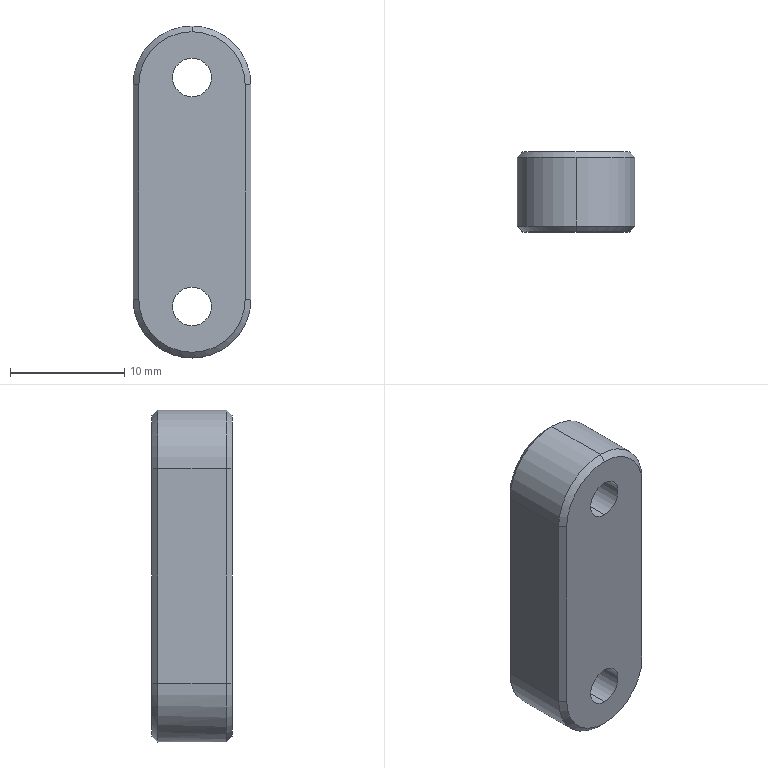Part | SolidWorks | features Fillet 2, ICE 2, Chamfer 1, Extrusion 1, HoleWzd 1 | 1 solid | 27 faces | box 10.3 x 7 x 29 mm | volume 1657 mm3 | cylinder 11 | plane 10 | cone 6 | commonest cylinder face diameters 3.4 x4 6 x4 10.3 x3
STEP:
#1=CARTESIAN_POINT('',(0.,0.1,21.5));
#2=VERTEX_POINT('',#1);
#3=CARTESIAN_POINT('',(0.,0.1,27.5));
#4=VERTEX_POINT('',#3);
#5=CARTESIAN_POINT('',(0.,0.1,24.5));
#6=DIRECTION('',(0.,1.,0.));
#7=DIRECTION('',(0.,0.,1.));
#8=AXIS2_PLACEMENT_3D('',#5,#6,#7);
#9=CIRCLE('',#8,3.);
#10=EDGE_CURVE('',#2,#4,#9,.T.);
#11=ORIENTED_EDGE('',*,*,#10,.F.);
#12=CARTESIAN_POINT('',(0.,3.5,21.5));
#13=VERTEX_POINT('',#12);
#14=CARTESIAN_POINT('',(0.,3.5,21.5));
#15=DIRECTION('',(0.,1.,0.));
#16=VECTOR('',#15,1000.);
#17=LINE('',#14,#16);
#18=EDGE_CURVE('',#2,#13,#17,.T.);
#19=ORIENTED_EDGE('',*,*,#18,.T.);
#20=CARTESIAN_POINT('',(0.,3.5,27.5));
#21=VERTEX_POINT('',#20);
#22=CARTESIAN_POINT('',(0.,3.5,24.5));
#23=DIRECTION('',(0.,1.,0.));
#24=DIRECTION('',(0.,0.,1.));
#25=AXIS2_PLACEMENT_3D('',#22,#23,#24);
#26=CIRCLE('',#25,3.);
#27=EDGE_CURVE('',#13,#21,#26,.T.);
#28=ORIENTED_EDGE('',*,*,#27,.T.);
#29=CARTESIAN_POINT('',(0.,3.5,27.5));
#30=DIRECTION('',(0.,1.,0.));
#31=VECTOR('',#30,1000.);
#32=LINE('',#29,#31);
#33=EDGE_CURVE('',#4,#21,#32,.T.);
#34=ORIENTED_EDGE('',*,*,#33,.F.);
#35=EDGE_LOOP('',(#11,#19,#28,#34));
#36=FACE_OUTER_BOUND('',#35,.T.);
#37=CARTESIAN_POINT('',(0.,3.5,24.5));
#38=DIRECTION('',(0.,1.,0.));
#39=DIRECTION('',(0.,0.,1.));
#40=AXIS2_PLACEMENT_3D('',#37,#38,#39);
#41=CYLINDRICAL_SURFACE('',#40,3.);
#42=ADVANCED_FACE('',(#36),#41,.F.);
#43=CARTESIAN_POINT('',(0.,-3.5,22.8));
#44=VERTEX_POINT('',#43);
#45=CARTESIAN_POINT('',(0.,-3.5,26.2));
#46=VERTEX_POINT('',#45);
#47=CARTESIAN_POINT('',(0.,-3.5,24.5));
#48=DIRECTION('',(0.,1.,0.));
#49=DIRECTION('',(0.,0.,1.));
#50=AXIS2_PLACEMENT_3D('',#47,#48,#49);
#51=CIRCLE('',#50,1.7);
#52=EDGE_CURVE('',#44,#46,#51,.T.);
#53=ORIENTED_EDGE('',*,*,#52,.F.);
#54=CARTESIAN_POINT('',(0.,0.1,22.8));
#55=VERTEX_POINT('',#54);
#56=CARTESIAN_POINT('',(0.,3.5,22.8));
#57=DIRECTION('',(0.,1.,0.));
#58=VECTOR('',#57,1000.);
#59=LINE('',#56,#58);
#60=EDGE_CURVE('',#44,#55,#59,.T.);
#61=ORIENTED_EDGE('',*,*,#60,.T.);
#62=CARTESIAN_POINT('',(0.,0.1,26.2));
#63=VERTEX_POINT('',#62);
#64=CARTESIAN_POINT('',(0.,0.1,24.5));
#65=DIRECTION('',(0.,1.,0.));
#66=DIRECTION('',(0.,0.,1.));
#67=AXIS2_PLACEMENT_3D('',#64,#65,#66);
#68=CIRCLE('',#67,1.7);
#69=EDGE_CURVE('',#55,#63,#68,.T.);
#70=ORIENTED_EDGE('',*,*,#69,.T.);
#71=CARTESIAN_POINT('',(0.,3.5,26.2));
#72=DIRECTION('',(0.,1.,0.));
#73=VECTOR('',#72,1000.);
#74=LINE('',#71,#73);
#75=EDGE_CURVE('',#46,#63,#74,.T.);
#76=ORIENTED_EDGE('',*,*,#75,.F.);
#77=EDGE_LOOP('',(#53,#61,#70,#76));
#78=FACE_OUTER_BOUND('',#77,.T.);
#79=CARTESIAN_POINT('',(0.,3.5,24.5));
#80=DIRECTION('',(0.,1.,0.));
#81=DIRECTION('',(0.,0.,1.));
#82=AXIS2_PLACEMENT_3D('',#79,#80,#81);
#83=CYLINDRICAL_SURFACE('',#82,1.7);
#84=ADVANCED_FACE('',(#78),#83,.F.);
#85=CARTESIAN_POINT('',(0.,0.1,1.5));
#86=VERTEX_POINT('',#85);
#87=CARTESIAN_POINT('',(0.,0.1,7.5));
#88=VERTEX_POINT('',#87);
#89=CARTESIAN_POINT('',(0.,0.1,4.5));
#90=DIRECTION('',(0.,1.,0.));
#91=DIRECTION('',(0.,0.,1.));
#92=AXIS2_PLACEMENT_3D('',#89,#90,#91);
#93=CIRCLE('',#92,3.);
#94=EDGE_CURVE('',#86,#88,#93,.T.);
#95=ORIENTED_EDGE('',*,*,#94,.F.);
#96=CARTESIAN_POINT('',(0.,3.5,1.5));
#97=VERTEX_POINT('',#96);
#98=CARTESIAN_POINT('',(0.,3.5,1.5));
#99=DIRECTION('',(0.,1.,0.));
#100=VECTOR('',#99,1000.);
#101=LINE('',#98,#100);
#102=EDGE_CURVE('',#86,#97,#101,.T.);
#103=ORIENTED_EDGE('',*,*,#102,.T.);
#104=CARTESIAN_POINT('',(0.,3.5,7.5));
#105=VERTEX_POINT('',#104);
#106=CARTESIAN_POINT('',(0.,3.5,4.5));
#107=DIRECTION('',(0.,1.,0.));
#108=DIRECTION('',(0.,0.,1.));
#109=AXIS2_PLACEMENT_3D('',#106,#107,#108);
#110=CIRCLE('',#109,3.);
#111=EDGE_CURVE('',#97,#105,#110,.T.);
#112=ORIENTED_EDGE('',*,*,#111,.T.);
#113=CARTESIAN_POINT('',(0.,3.5,7.5));
#114=DIRECTION('',(0.,1.,0.));
#115=VECTOR('',#114,1000.);
#116=LINE('',#113,#115);
#117=EDGE_CURVE('',#88,#105,#116,.T.);
#118=ORIENTED_EDGE('',*,*,#117,.F.);
#119=EDGE_LOOP('',(#95,#103,#112,#118));
#120=FACE_OUTER_BOUND('',#119,.T.);
#121=CARTESIAN_POINT('',(0.,3.5,4.5));
#122=DIRECTION('',(0.,1.,0.));
#123=DIRECTION('',(0.,0.,1.));
#124=AXIS2_PLACEMENT_3D('',#121,#122,#123);
#125=CYLINDRICAL_SURFACE('',#124,3.);
#126=ADVANCED_FACE('',(#120),#125,.F.);
#127=CARTESIAN_POINT('',(0.,-3.5,2.8));
#128=VERTEX_POINT('',#127);
#129=CARTESIAN_POINT('',(0.,-3.5,6.2));
#130=VERTEX_POINT('',#129);
#131=CARTESIAN_POINT('',(0.,-3.5,4.5));
#132=DIRECTION('',(0.,1.,0.));
#133=DIRECTION('',(0.,0.,1.));
#134=AXIS2_PLACEMENT_3D('',#131,#132,#133);
#135=CIRCLE('',#134,1.7);
#136=EDGE_CURVE('',#128,#130,#135,.T.);
#137=ORIENTED_EDGE('',*,*,#136,.F.);
#138=CARTESIAN_POINT('',(0.,0.1,2.8));
#139=VERTEX_POINT('',#138);
#140=CARTESIAN_POINT('',(0.,3.5,2.8));
#141=DIRECTION('',(0.,1.,0.));
#142=VECTOR('',#141,1000.);
#143=LINE('',#140,#142);
#144=EDGE_CURVE('',#128,#139,#143,.T.);
#145=ORIENTED_EDGE('',*,*,#144,.T.);
#146=CARTESIAN_POINT('',(0.,0.1,6.2));
#147=VERTEX_POINT('',#146);
#148=CARTESIAN_POINT('',(0.,0.1,4.5));
#149=DIRECTION('',(0.,1.,0.));
#150=DIRECTION('',(0.,0.,1.));
#151=AXIS2_PLACEMENT_3D('',#148,#149,#150);
#152=CIRCLE('',#151,1.7);
#153=EDGE_CURVE('',#139,#147,#152,.T.);
#154=ORIENTED_EDGE('',*,*,#153,.T.);
#155=CARTESIAN_POINT('',(0.,3.5,6.2));
#156=DIRECTION('',(0.,1.,0.));
#157=VECTOR('',#156,1000.);
#158=LINE('',#155,#157);
#159=EDGE_CURVE('',#130,#147,#158,.T.);
#160=ORIENTED_EDGE('',*,*,#159,.F.);
#161=EDGE_LOOP('',(#137,#145,#154,#160));
#162=FACE_OUTER_BOUND('',#161,.T.);
#163=CARTESIAN_POINT('',(0.,3.5,4.5));
#164=DIRECTION('',(0.,1.,0.));
#165=DIRECTION('',(0.,0.,1.));
#166=AXIS2_PLACEMENT_3D('',#163,#164,#165);
#167=CYLINDRICAL_SURFACE('',#166,1.7);
#168=ADVANCED_FACE('',(#162),#167,.F.);
#169=CARTESIAN_POINT('',(0.,3.5,0.5));
#170=VERTEX_POINT('',#169);
#171=CARTESIAN_POINT('',(-4.65,3.5,5.15));
#172=VERTEX_POINT('',#171);
#173=CARTESIAN_POINT('',(0.,3.5,5.15));
#174=DIRECTION('',(0.,1.,0.));
#175=DIRECTION('',(0.,0.,-1.));
#176=AXIS2_PLACEMENT_3D('',#173,#174,#175);
#177=CIRCLE('',#176,4.65);
#178=EDGE_CURVE('',#170,#172,#177,.T.);
#179=ORIENTED_EDGE('',*,*,#178,.F.);
#180=CARTESIAN_POINT('',(0.,3.,0.));
#181=VERTEX_POINT('',#180);
#182=CARTESIAN_POINT('',(0.,3.5,0.5));
#183=DIRECTION('',(0.,-0.7071,-0.7071));
#184=VECTOR('',#183,1000.);
#185=LINE('',#182,#184);
#186=EDGE_CURVE('',#170,#181,#185,.T.);
#187=ORIENTED_EDGE('',*,*,#186,.T.);
#188=CARTESIAN_POINT('',(-5.15,3.,5.15));
#189=VERTEX_POINT('',#188);
#190=CARTESIAN_POINT('',(0.,3.,5.15));
#191=DIRECTION('',(0.,-1.,0.));
#192=DIRECTION('',(0.,0.,-1.));
#193=AXIS2_PLACEMENT_3D('',#190,#191,#192);
#194=CIRCLE('',#193,5.15);
#195=EDGE_CURVE('',#189,#181,#194,.T.);
#196=ORIENTED_EDGE('',*,*,#195,.F.);
#197=CARTESIAN_POINT('',(-5.15,3.,5.15));
#198=DIRECTION('',(0.7071,0.7071,0.));
#199=VECTOR('',#198,1000.);
#200=LINE('',#197,#199);
#201=EDGE_CURVE('',#189,#172,#200,.T.);
#202=ORIENTED_EDGE('',*,*,#201,.T.);
#203=EDGE_LOOP('',(#179,#187,#196,#202));
#204=FACE_OUTER_BOUND('',#203,.T.);
#205=CARTESIAN_POINT('',(0.,3.5,5.15));
#206=DIRECTION('',(0.,-1.,0.));
#207=DIRECTION('',(0.,0.,-1.));
#208=AXIS2_PLACEMENT_3D('',#205,#206,#207);
#209=CONICAL_SURFACE('',#208,4.65,0.7854);
#210=ADVANCED_FACE('',(#204),#209,.T.);
#211=CARTESIAN_POINT('',(0.,-3.5,28.5));
#212=VERTEX_POINT('',#211);
#213=CARTESIAN_POINT('',(-4.65,-3.5,23.85));
#214=VERTEX_POINT('',#213);
#215=CARTESIAN_POINT('',(0.,-3.5,23.85));
#216=DIRECTION('',(0.,-1.,0.));
#217=DIRECTION('',(0.,0.,1.));
#218=AXIS2_PLACEMENT_3D('',#215,#216,#217);
#219=CIRCLE('',#218,4.65);
#220=EDGE_CURVE('',#212,#214,#219,.T.);
#221=ORIENTED_EDGE('',*,*,#220,.F.);
#222=CARTESIAN_POINT('',(0.,-3.,29.));
#223=VERTEX_POINT('',#222);
#224=CARTESIAN_POINT('',(0.,-3.5,28.5));
#225=DIRECTION('',(0.,0.7071,0.7071));
#226=VECTOR('',#225,1000.);
#227=LINE('',#224,#226);
#228=EDGE_CURVE('',#212,#223,#227,.T.);
#229=ORIENTED_EDGE('',*,*,#228,.T.);
#230=CARTESIAN_POINT('',(-5.15,-3.,23.85));
#231=VERTEX_POINT('',#230);
#232=CARTESIAN_POINT('',(0.,-3.,23.85));
#233=DIRECTION('',(0.,1.,0.));
#234=DIRECTION('',(0.,0.,1.));
#235=AXIS2_PLACEMENT_3D('',#232,#233,#234);
#236=CIRCLE('',#235,5.15);
#237=EDGE_CURVE('',#231,#223,#236,.T.);
#238=ORIENTED_EDGE('',*,*,#237,.F.);
#239=CARTESIAN_POINT('',(-5.15,-3.,23.85));
#240=DIRECTION('',(0.7071,-0.7071,0.));
#241=VECTOR('',#240,1000.);
#242=LINE('',#239,#241);
#243=EDGE_CURVE('',#231,#214,#242,.T.);
#244=ORIENTED_EDGE('',*,*,#243,.T.);
#245=EDGE_LOOP('',(#221,#229,#238,#244));
#246=FACE_OUTER_BOUND('',#245,.T.);
#247=CARTESIAN_POINT('',(0.,-3.5,23.85));
#248=DIRECTION('',(0.,1.,0.));
#249=DIRECTION('',(0.,0.,1.));
#250=AXIS2_PLACEMENT_3D('',#247,#248,#249);
#251=CONICAL_SURFACE('',#250,4.65,0.7854);
#252=ADVANCED_FACE('',(#246),#251,.T.);
#253=ORIENTED_EDGE('',*,*,#237,.T.);
#254=CARTESIAN_POINT('',(0.,3.,29.));
#255=VERTEX_POINT('',#254);
#256=CARTESIAN_POINT('',(0.,3.5,29.));
#257=DIRECTION('',(0.,1.,0.));
#258=VECTOR('',#257,1000.);
#259=LINE('',#256,#258);
#260=EDGE_CURVE('',#223,#255,#259,.T.);
#261=ORIENTED_EDGE('',*,*,#260,.T.);
#262=CARTESIAN_POINT('',(-5.15,3.,23.85));
#263=VERTEX_POINT('',#262);
#264=CARTESIAN_POINT('',(0.,3.,23.85));
#265=DIRECTION('',(0.,-1.,0.));
#266=DIRECTION('',(0.,0.,-1.));
#267=AXIS2_PLACEMENT_3D('',#264,#265,#266);
#268=CIRCLE('',#267,5.15);
#269=EDGE_CURVE('',#255,#263,#268,.T.);
#270=ORIENTED_EDGE('',*,*,#269,.T.);
#271=CARTESIAN_POINT('',(-5.15,3.5,23.85));
#272=DIRECTION('',(0.,1.,0.));
#273=VECTOR('',#272,1000.);
#274=LINE('',#271,#273);
#275=EDGE_CURVE('',#231,#263,#274,.T.);
#276=ORIENTED_EDGE('',*,*,#275,.F.);
#277=EDGE_LOOP('',(#253,#261,#270,#276));
#278=FACE_OUTER_BOUND('',#277,.T.);
#279=CARTESIAN_POINT('',(0.,3.5,23.85));
#280=DIRECTION('',(0.,1.,0.));
#281=DIRECTION('',(0.,0.,1.));
#282=AXIS2_PLACEMENT_3D('',#279,#280,#281);
#283=CYLINDRICAL_SURFACE('',#282,5.15);
#284=ADVANCED_FACE('',(#278),#283,.T.);
#285=ORIENTED_EDGE('',*,*,#260,.F.);
#286=CARTESIAN_POINT('',(5.15,-3.,23.85));
#287=VERTEX_POINT('',#286);
#288=CARTESIAN_POINT('',(0.,-3.,23.85));
#289=DIRECTION('',(0.,1.,0.));
#290=DIRECTION('',(0.,0.,1.));
#291=AXIS2_PLACEMENT_3D('',#288,#289,#290);
#292=CIRCLE('',#291,5.15);
#293=EDGE_CURVE('',#223,#287,#292,.T.);
#294=ORIENTED_EDGE('',*,*,#293,.T.);
#295=CARTESIAN_POINT('',(5.15,3.,23.85));
#296=VERTEX_POINT('',#295);
#297=CARTESIAN_POINT('',(5.15,3.5,23.85));
#298=DIRECTION('',(0.,-1.,0.));
#299=VECTOR('',#298,1000.);
#300=LINE('',#297,#299);
#301=EDGE_CURVE('',#296,#287,#300,.T.);
#302=ORIENTED_EDGE('',*,*,#301,.F.);
#303=CARTESIAN_POINT('',(0.,3.,23.85));
#304=DIRECTION('',(0.,-1.,0.));
#305=DIRECTION('',(0.,0.,-1.));
#306=AXIS2_PLACEMENT_3D('',#303,#304,#305);
#307=CIRCLE('',#306,5.15);
#308=EDGE_CURVE('',#296,#255,#307,.T.);
#309=ORIENTED_EDGE('',*,*,#308,.T.);
#310=EDGE_LOOP('',(#285,#294,#302,#309));
#311=FACE_OUTER_BOUND('',#310,.T.);
#312=CARTESIAN_POINT('',(0.,3.5,23.85));
#313=DIRECTION('',(0.,1.,0.));
#314=DIRECTION('',(0.,0.,1.));
#315=AXIS2_PLACEMENT_3D('',#312,#313,#314);
#316=CYLINDRICAL_SURFACE('',#315,5.15);
#317=ADVANCED_FACE('',(#311),#316,.T.);
#318=CARTESIAN_POINT('',(5.15,-3.,5.15));
#319=VERTEX_POINT('',#318);
#320=CARTESIAN_POINT('',(5.15,3.,5.15));
#321=VERTEX_POINT('',#320);
#322=CARTESIAN_POINT('',(5.15,3.5,5.15));
#323=DIRECTION('',(0.,1.,0.));
#324=VECTOR('',#323,1000.);
#325=LINE('',#322,#324);
#326=EDGE_CURVE('',#319,#321,#325,.T.);
#327=ORIENTED_EDGE('',*,*,#326,.F.);
#328=CARTESIAN_POINT('',(-5.15,-3.,5.15));
#329=VERTEX_POINT('',#328);
#330=CARTESIAN_POINT('',(0.,-3.,5.15));
#331=DIRECTION('',(0.,1.,0.));
#332=DIRECTION('',(0.,0.,1.));
#333=AXIS2_PLACEMENT_3D('',#330,#331,#332);
#334=CIRCLE('',#333,5.15);
#335=EDGE_CURVE('',#319,#329,#334,.T.);
#336=ORIENTED_EDGE('',*,*,#335,.T.);
#337=CARTESIAN_POINT('',(-5.15,3.5,5.15));
#338=DIRECTION('',(0.,-1.,0.));
#339=VECTOR('',#338,1000.);
#340=LINE('',#337,#339);
#341=EDGE_CURVE('',#189,#329,#340,.T.);
#342=ORIENTED_EDGE('',*,*,#341,.F.);
#343=ORIENTED_EDGE('',*,*,#195,.T.);
#344=CARTESIAN_POINT('',(0.,3.,5.15));
#345=DIRECTION('',(0.,-1.,0.));
#346=DIRECTION('',(0.,0.,-1.));
#347=AXIS2_PLACEMENT_3D('',#344,#345,#346);
#348=CIRCLE('',#347,5.15);
#349=EDGE_CURVE('',#181,#321,#348,.T.);
#350=ORIENTED_EDGE('',*,*,#349,.T.);
#351=EDGE_LOOP('',(#327,#336,#342,#343,#350));
#352=FACE_OUTER_BOUND('',#351,.T.);
#353=CARTESIAN_POINT('',(0.,-3.5,5.15));
#354=DIRECTION('',(0.,1.,0.));
#355=DIRECTION('',(0.,0.,1.));
#356=AXIS2_PLACEMENT_3D('',#353,#354,#355);
#357=CYLINDRICAL_SURFACE('',#356,5.15);
#358=ADVANCED_FACE('',(#352),#357,.T.);
#359=ORIENTED_EDGE('',*,*,#301,.T.);
#360=CARTESIAN_POINT('',(5.15,-3.,29.));
#361=DIRECTION('',(0.,0.,-1.));
#362=VECTOR('',#361,1000.);
#363=LINE('',#360,#362);
#364=EDGE_CURVE('',#287,#319,#363,.T.);
#365=ORIENTED_EDGE('',*,*,#364,.T.);
#366=ORIENTED_EDGE('',*,*,#326,.T.);
#367=CARTESIAN_POINT('',(5.15,3.,29.));
#368=DIRECTION('',(0.,0.,1.));
#369=VECTOR('',#368,1000.);
#370=LINE('',#367,#369);
#371=EDGE_CURVE('',#321,#296,#370,.T.);
#372=ORIENTED_EDGE('',*,*,#371,.T.);
#373=EDGE_LOOP('',(#359,#365,#366,#372));
#374=FACE_OUTER_BOUND('',#373,.T.);
#375=CARTESIAN_POINT('',(5.15,3.5,29.));
#376=DIRECTION('',(-1.,0.,0.));
#377=DIRECTION('',(0.,0.,1.));
#378=AXIS2_PLACEMENT_3D('',#375,#376,#377);
#379=PLANE('',#378);
#380=ADVANCED_FACE('',(#374),#379,.F.);
#381=CARTESIAN_POINT('',(0.,3.5,24.5));
#382=DIRECTION('',(0.,1.,0.));
#383=DIRECTION('',(0.,0.,1.));
#384=AXIS2_PLACEMENT_3D('',#381,#382,#383);
#385=CIRCLE('',#384,3.);
#386=EDGE_CURVE('',#21,#13,#385,.T.);
#387=ORIENTED_EDGE('',*,*,#386,.F.);
#388=ORIENTED_EDGE('',*,*,#27,.F.);
#389=EDGE_LOOP('',(#387,#388));
#390=FACE_BOUND('',#389,.T.);
#391=CARTESIAN_POINT('',(0.,3.5,4.5));
#392=DIRECTION('',(0.,1.,0.));
#393=DIRECTION('',(0.,0.,1.));
#394=AXIS2_PLACEMENT_3D('',#391,#392,#393);
#395=CIRCLE('',#394,3.);
#396=EDGE_CURVE('',#105,#97,#395,.T.);
#397=ORIENTED_EDGE('',*,*,#396,.F.);
#398=ORIENTED_EDGE('',*,*,#111,.F.);
#399=EDGE_LOOP('',(#397,#398));
#400=FACE_BOUND('',#399,.T.);
#401=CARTESIAN_POINT('',(-4.65,3.5,23.85));
#402=VERTEX_POINT('',#401);
#403=CARTESIAN_POINT('',(4.65,3.5,23.85));
#404=VERTEX_POINT('',#403);
#405=CARTESIAN_POINT('',(0.,3.5,23.85));
#406=DIRECTION('',(0.,1.,0.));
#407=DIRECTION('',(0.,0.,-1.));
#408=AXIS2_PLACEMENT_3D('',#405,#406,#407);
#409=CIRCLE('',#408,4.65);
#410=EDGE_CURVE('',#402,#404,#409,.T.);
#411=ORIENTED_EDGE('',*,*,#410,.T.);
#412=CARTESIAN_POINT('',(4.65,3.5,5.15));
#413=VERTEX_POINT('',#412);
#414=CARTESIAN_POINT('',(4.65,3.5,29.));
#415=DIRECTION('',(0.,0.,-1.));
#416=VECTOR('',#415,1000.);
#417=LINE('',#414,#416);
#418=EDGE_CURVE('',#404,#413,#417,.T.);
#419=ORIENTED_EDGE('',*,*,#418,.T.);
#420=CARTESIAN_POINT('',(0.,3.5,5.15));
#421=DIRECTION('',(0.,1.,0.));
#422=DIRECTION('',(0.,0.,-1.));
#423=AXIS2_PLACEMENT_3D('',#420,#421,#422);
#424=CIRCLE('',#423,4.65);
#425=EDGE_CURVE('',#413,#170,#424,.T.);
#426=ORIENTED_EDGE('',*,*,#425,.T.);
#427=ORIENTED_EDGE('',*,*,#178,.T.);
#428=CARTESIAN_POINT('',(-4.65,3.5,29.));
#429=DIRECTION('',(0.,0.,1.));
#430=VECTOR('',#429,1000.);
#431=LINE('',#428,#430);
#432=EDGE_CURVE('',#172,#402,#431,.T.);
#433=ORIENTED_EDGE('',*,*,#432,.T.);
#434=EDGE_LOOP('',(#411,#419,#426,#427,#433));
#435=FACE_OUTER_BOUND('',#434,.T.);
#436=CARTESIAN_POINT('',(-5.15,3.5,29.));
#437=DIRECTION('',(0.,-1.,0.));
#438=DIRECTION('',(0.,0.,-1.));
#439=AXIS2_PLACEMENT_3D('',#436,#437,#438);
#440=PLANE('',#439);
#441=ADVANCED_FACE('',(#390,#400,#435),#440,.F.);
#442=ORIENTED_EDGE('',*,*,#341,.T.);
#443=CARTESIAN_POINT('',(-5.15,-3.,29.));
#444=DIRECTION('',(0.,0.,1.));
#445=VECTOR('',#444,1000.);
#446=LINE('',#443,#445);
#447=EDGE_CURVE('',#329,#231,#446,.T.);
#448=ORIENTED_EDGE('',*,*,#447,.T.);
#449=ORIENTED_EDGE('',*,*,#275,.T.);
#450=CARTESIAN_POINT('',(-5.15,3.,29.));
#451=DIRECTION('',(0.,0.,-1.));
#452=VECTOR('',#451,1000.);
#453=LINE('',#450,#452);
#454=EDGE_CURVE('',#263,#189,#453,.T.);
#455=ORIENTED_EDGE('',*,*,#454,.T.);
#456=EDGE_LOOP('',(#442,#448,#449,#455));
#457=FACE_OUTER_BOUND('',#456,.T.);
#458=CARTESIAN_POINT('',(-5.15,3.5,29.));
#459=DIRECTION('',(1.,0.,0.));
#460=DIRECTION('',(0.,1.,0.));
#461=AXIS2_PLACEMENT_3D('',#458,#459,#460);
#462=PLANE('',#461);
#463=ADVANCED_FACE('',(#457),#462,.F.);
#464=CARTESIAN_POINT('',(0.,-3.5,24.5));
#465=DIRECTION('',(0.,1.,0.));
#466=DIRECTION('',(0.,0.,1.));
#467=AXIS2_PLACEMENT_3D('',#464,#465,#466);
#468=CIRCLE('',#467,1.7);
#469=EDGE_CURVE('',#46,#44,#468,.T.);
#470=ORIENTED_EDGE('',*,*,#469,.T.);
#471=ORIENTED_EDGE('',*,*,#52,.T.);
#472=EDGE_LOOP('',(#470,#471));
#473=FACE_BOUND('',#472,.T.);
#474=CARTESIAN_POINT('',(0.,-3.5,4.5));
#475=DIRECTION('',(0.,1.,0.));
#476=DIRECTION('',(0.,0.,1.));
#477=AXIS2_PLACEMENT_3D('',#474,#475,#476);
#478=CIRCLE('',#477,1.7);
#479=EDGE_CURVE('',#130,#128,#478,.T.);
#480=ORIENTED_EDGE('',*,*,#479,.T.);
#481=ORIENTED_EDGE('',*,*,#136,.T.);
#482=EDGE_LOOP('',(#480,#481));
#483=FACE_BOUND('',#482,.T.);
#484=CARTESIAN_POINT('',(-4.65,-3.5,5.15));
#485=VERTEX_POINT('',#484);
#486=CARTESIAN_POINT('',(4.65,-3.5,5.15));
#487=VERTEX_POINT('',#486);
#488=CARTESIAN_POINT('',(0.,-3.5,5.15));
#489=DIRECTION('',(0.,-1.,0.));
#490=DIRECTION('',(0.,0.,1.));
#491=AXIS2_PLACEMENT_3D('',#488,#489,#490);
#492=CIRCLE('',#491,4.65);
#493=EDGE_CURVE('',#485,#487,#492,.T.);
#494=ORIENTED_EDGE('',*,*,#493,.T.);
#495=CARTESIAN_POINT('',(4.65,-3.5,23.85));
#496=VERTEX_POINT('',#495);
#497=CARTESIAN_POINT('',(4.65,-3.5,29.));
#498=DIRECTION('',(0.,0.,1.));
#499=VECTOR('',#498,1000.);
#500=LINE('',#497,#499);
#501=EDGE_CURVE('',#487,#496,#500,.T.);
#502=ORIENTED_EDGE('',*,*,#501,.T.);
#503=CARTESIAN_POINT('',(0.,-3.5,23.85));
#504=DIRECTION('',(0.,-1.,0.));
#505=DIRECTION('',(0.,0.,1.));
#506=AXIS2_PLACEMENT_3D('',#503,#504,#505);
#507=CIRCLE('',#506,4.65);
#508=EDGE_CURVE('',#496,#212,#507,.T.);
#509=ORIENTED_EDGE('',*,*,#508,.T.);
#510=ORIENTED_EDGE('',*,*,#220,.T.);
#511=CARTESIAN_POINT('',(-4.65,-3.5,29.));
#512=DIRECTION('',(0.,0.,-1.));
#513=VECTOR('',#512,1000.);
#514=LINE('',#511,#513);
#515=EDGE_CURVE('',#214,#485,#514,.T.);
#516=ORIENTED_EDGE('',*,*,#515,.T.);
#517=EDGE_LOOP('',(#494,#502,#509,#510,#516));
#518=FACE_OUTER_BOUND('',#517,.T.);
#519=CARTESIAN_POINT('',(-5.15,-3.5,29.));
#520=DIRECTION('',(0.,1.,0.));
#521=DIRECTION('',(0.,0.,1.));
#522=AXIS2_PLACEMENT_3D('',#519,#520,#521);
#523=PLANE('',#522);
#524=ADVANCED_FACE('',(#473,#483,#518),#523,.F.);
#525=CARTESIAN_POINT('',(-4.65,-3.5,5.15));
#526=DIRECTION('',(-0.7071,0.7071,0.));
#527=VECTOR('',#526,1000.);
#528=LINE('',#525,#527);
#529=EDGE_CURVE('',#485,#329,#528,.T.);
#530=ORIENTED_EDGE('',*,*,#529,.F.);
#531=ORIENTED_EDGE('',*,*,#515,.F.);
#532=ORIENTED_EDGE('',*,*,#243,.F.);
#533=ORIENTED_EDGE('',*,*,#447,.F.);
#534=EDGE_LOOP('',(#530,#531,#532,#533));
#535=FACE_OUTER_BOUND('',#534,.T.);
#536=CARTESIAN_POINT('',(-4.65,-3.5,29.));
#537=DIRECTION('',(0.7071,0.7071,0.));
#538=DIRECTION('',(0.,0.,-1.));
#539=AXIS2_PLACEMENT_3D('',#536,#537,#538);
#540=PLANE('',#539);
#541=ADVANCED_FACE('',(#535),#540,.F.);
#542=ORIENTED_EDGE('',*,*,#228,.F.);
#543=ORIENTED_EDGE('',*,*,#508,.F.);
#544=CARTESIAN_POINT('',(5.15,-3.,23.85));
#545=DIRECTION('',(-0.7071,-0.7071,0.));
#546=VECTOR('',#545,1000.);
#547=LINE('',#544,#546);
#548=EDGE_CURVE('',#287,#496,#547,.T.);
#549=ORIENTED_EDGE('',*,*,#548,.F.);
#550=ORIENTED_EDGE('',*,*,#293,.F.);
#551=EDGE_LOOP('',(#542,#543,#549,#550));
#552=FACE_OUTER_BOUND('',#551,.T.);
#553=CARTESIAN_POINT('',(0.,-3.5,23.85));
#554=DIRECTION('',(0.,1.,0.));
#555=DIRECTION('',(0.,0.,1.));
#556=AXIS2_PLACEMENT_3D('',#553,#554,#555);
#557=CONICAL_SURFACE('',#556,4.65,0.7854);
#558=ADVANCED_FACE('',(#552),#557,.T.);
#559=ORIENTED_EDGE('',*,*,#529,.T.);
#560=ORIENTED_EDGE('',*,*,#335,.F.);
#561=CARTESIAN_POINT('',(4.65,-3.5,5.15));
#562=DIRECTION('',(0.7071,0.7071,0.));
#563=VECTOR('',#562,1000.);
#564=LINE('',#561,#563);
#565=EDGE_CURVE('',#487,#319,#564,.T.);
#566=ORIENTED_EDGE('',*,*,#565,.F.);
#567=ORIENTED_EDGE('',*,*,#493,.F.);
#568=EDGE_LOOP('',(#559,#560,#566,#567));
#569=FACE_OUTER_BOUND('',#568,.T.);
#570=CARTESIAN_POINT('',(0.,-3.5,5.15));
#571=DIRECTION('',(0.,1.,0.));
#572=DIRECTION('',(0.,0.,1.));
#573=AXIS2_PLACEMENT_3D('',#570,#571,#572);
#574=CONICAL_SURFACE('',#573,4.65,0.7854);
#575=ADVANCED_FACE('',(#569),#574,.T.);
#576=ORIENTED_EDGE('',*,*,#548,.T.);
#577=ORIENTED_EDGE('',*,*,#501,.F.);
#578=ORIENTED_EDGE('',*,*,#565,.T.);
#579=ORIENTED_EDGE('',*,*,#364,.F.);
#580=EDGE_LOOP('',(#576,#577,#578,#579));
#581=FACE_OUTER_BOUND('',#580,.T.);
#582=CARTESIAN_POINT('',(5.15,-3.,29.));
#583=DIRECTION('',(-0.7071,0.7071,0.));
#584=DIRECTION('',(0.,0.,-1.));
#585=AXIS2_PLACEMENT_3D('',#582,#583,#584);
#586=PLANE('',#585);
#587=ADVANCED_FACE('',(#581),#586,.F.);
#588=ORIENTED_EDGE('',*,*,#201,.F.);
#589=ORIENTED_EDGE('',*,*,#454,.F.);
#590=CARTESIAN_POINT('',(-4.65,3.5,23.85));
#591=DIRECTION('',(-0.7071,-0.7071,0.));
#592=VECTOR('',#591,1000.);
#593=LINE('',#590,#592);
#594=EDGE_CURVE('',#402,#263,#593,.T.);
#595=ORIENTED_EDGE('',*,*,#594,.F.);
#596=ORIENTED_EDGE('',*,*,#432,.F.);
#597=EDGE_LOOP('',(#588,#589,#595,#596));
#598=FACE_OUTER_BOUND('',#597,.T.);
#599=CARTESIAN_POINT('',(-5.15,3.,29.));
#600=DIRECTION('',(0.7071,-0.7071,0.));
#601=DIRECTION('',(0.,0.,-1.));
#602=AXIS2_PLACEMENT_3D('',#599,#600,#601);
#603=PLANE('',#602);
#604=ADVANCED_FACE('',(#598),#603,.F.);
#605=ORIENTED_EDGE('',*,*,#594,.T.);
#606=ORIENTED_EDGE('',*,*,#269,.F.);
#607=ORIENTED_EDGE('',*,*,#308,.F.);
#608=CARTESIAN_POINT('',(4.65,3.5,23.85));
#609=DIRECTION('',(0.7071,-0.7071,0.));
#610=VECTOR('',#609,1000.);
#611=LINE('',#608,#610);
#612=EDGE_CURVE('',#404,#296,#611,.T.);
#613=ORIENTED_EDGE('',*,*,#612,.F.);
#614=ORIENTED_EDGE('',*,*,#410,.F.);
#615=EDGE_LOOP('',(#605,#606,#607,#613,#614));
#616=FACE_OUTER_BOUND('',#615,.T.);
#617=CARTESIAN_POINT('',(0.,3.5,23.85));
#618=DIRECTION('',(0.,-1.,0.));
#619=DIRECTION('',(0.,0.,-1.));
#620=AXIS2_PLACEMENT_3D('',#617,#618,#619);
#621=CONICAL_SURFACE('',#620,4.65,0.7854);
#622=ADVANCED_FACE('',(#616),#621,.T.);
#623=ORIENTED_EDGE('',*,*,#186,.F.);
#624=ORIENTED_EDGE('',*,*,#425,.F.);
#625=CARTESIAN_POINT('',(5.15,3.,5.15));
#626=DIRECTION('',(-0.7071,0.7071,0.));
#627=VECTOR('',#626,1000.);
#628=LINE('',#625,#627);
#629=EDGE_CURVE('',#321,#413,#628,.T.);
#630=ORIENTED_EDGE('',*,*,#629,.F.);
#631=ORIENTED_EDGE('',*,*,#349,.F.);
#632=EDGE_LOOP('',(#623,#624,#630,#631));
#633=FACE_OUTER_BOUND('',#632,.T.);
#634=CARTESIAN_POINT('',(0.,3.5,5.15));
#635=DIRECTION('',(0.,-1.,0.));
#636=DIRECTION('',(0.,0.,-1.));
#637=AXIS2_PLACEMENT_3D('',#634,#635,#636);
#638=CONICAL_SURFACE('',#637,4.65,0.7854);
#639=ADVANCED_FACE('',(#633),#638,.T.);
#640=ORIENTED_EDGE('',*,*,#612,.T.);
#641=ORIENTED_EDGE('',*,*,#371,.F.);
#642=ORIENTED_EDGE('',*,*,#629,.T.);
#643=ORIENTED_EDGE('',*,*,#418,.F.);
#644=EDGE_LOOP('',(#640,#641,#642,#643));
#645=FACE_OUTER_BOUND('',#644,.T.);
#646=CARTESIAN_POINT('',(4.65,3.5,29.));
#647=DIRECTION('',(-0.7071,-0.7071,0.));
#648=DIRECTION('',(0.,0.,-1.));
#649=AXIS2_PLACEMENT_3D('',#646,#647,#648);
#650=PLANE('',#649);
#651=ADVANCED_FACE('',(#645),#650,.F.);
#652=ORIENTED_EDGE('',*,*,#144,.F.);
#653=ORIENTED_EDGE('',*,*,#479,.F.);
#654=ORIENTED_EDGE('',*,*,#159,.T.);
#655=CARTESIAN_POINT('',(0.,0.1,4.5));
#656=DIRECTION('',(0.,1.,0.));
#657=DIRECTION('',(0.,0.,1.));
#658=AXIS2_PLACEMENT_3D('',#655,#656,#657);
#659=CIRCLE('',#658,1.7);
#660=EDGE_CURVE('',#147,#139,#659,.T.);
#661=ORIENTED_EDGE('',*,*,#660,.T.);
#662=EDGE_LOOP('',(#652,#653,#654,#661));
#663=FACE_OUTER_BOUND('',#662,.T.);
#664=CARTESIAN_POINT('',(0.,3.5,4.5));
#665=DIRECTION('',(0.,1.,0.));
#666=DIRECTION('',(0.,0.,1.));
#667=AXIS2_PLACEMENT_3D('',#664,#665,#666);
#668=CYLINDRICAL_SURFACE('',#667,1.7);
#669=ADVANCED_FACE('',(#663),#668,.F.);
#670=ORIENTED_EDGE('',*,*,#660,.F.);
#671=ORIENTED_EDGE('',*,*,#153,.F.);
#672=EDGE_LOOP('',(#670,#671));
#673=FACE_BOUND('',#672,.T.);
#674=CARTESIAN_POINT('',(0.,0.1,4.5));
#675=DIRECTION('',(0.,1.,0.));
#676=DIRECTION('',(0.,0.,1.));
#677=AXIS2_PLACEMENT_3D('',#674,#675,#676);
#678=CIRCLE('',#677,3.);
#679=EDGE_CURVE('',#88,#86,#678,.T.);
#680=ORIENTED_EDGE('',*,*,#679,.T.);
#681=ORIENTED_EDGE('',*,*,#94,.T.);
#682=EDGE_LOOP('',(#680,#681));
#683=FACE_OUTER_BOUND('',#682,.T.);
#684=CARTESIAN_POINT('',(1.7,0.1,4.5));
#685=DIRECTION('',(0.,-1.,0.));
#686=DIRECTION('',(0.,0.,-1.));
#687=AXIS2_PLACEMENT_3D('',#684,#685,#686);
#688=PLANE('',#687);
#689=ADVANCED_FACE('',(#673,#683),#688,.F.);
#690=ORIENTED_EDGE('',*,*,#102,.F.);
#691=ORIENTED_EDGE('',*,*,#679,.F.);
#692=ORIENTED_EDGE('',*,*,#117,.T.);
#693=ORIENTED_EDGE('',*,*,#396,.T.);
#694=EDGE_LOOP('',(#690,#691,#692,#693));
#695=FACE_OUTER_BOUND('',#694,.T.);
#696=CARTESIAN_POINT('',(0.,3.5,4.5));
#697=DIRECTION('',(0.,1.,0.));
#698=DIRECTION('',(0.,0.,1.));
#699=AXIS2_PLACEMENT_3D('',#696,#697,#698);
#700=CYLINDRICAL_SURFACE('',#699,3.);
#701=ADVANCED_FACE('',(#695),#700,.F.);
#702=ORIENTED_EDGE('',*,*,#60,.F.);
#703=ORIENTED_EDGE('',*,*,#469,.F.);
#704=ORIENTED_EDGE('',*,*,#75,.T.);
#705=CARTESIAN_POINT('',(0.,0.1,24.5));
#706=DIRECTION('',(0.,1.,0.));
#707=DIRECTION('',(0.,0.,1.));
#708=AXIS2_PLACEMENT_3D('',#705,#706,#707);
#709=CIRCLE('',#708,1.7);
#710=EDGE_CURVE('',#63,#55,#709,.T.);
#711=ORIENTED_EDGE('',*,*,#710,.T.);
#712=EDGE_LOOP('',(#702,#703,#704,#711));
#713=FACE_OUTER_BOUND('',#712,.T.);
#714=CARTESIAN_POINT('',(0.,3.5,24.5));
#715=DIRECTION('',(0.,1.,0.));
#716=DIRECTION('',(0.,0.,1.));
#717=AXIS2_PLACEMENT_3D('',#714,#715,#716);
#718=CYLINDRICAL_SURFACE('',#717,1.7);
#719=ADVANCED_FACE('',(#713),#718,.F.);
#720=ORIENTED_EDGE('',*,*,#710,.F.);
#721=ORIENTED_EDGE('',*,*,#69,.F.);
#722=EDGE_LOOP('',(#720,#721));
#723=FACE_BOUND('',#722,.T.);
#724=CARTESIAN_POINT('',(0.,0.1,24.5));
#725=DIRECTION('',(0.,1.,0.));
#726=DIRECTION('',(0.,0.,1.));
#727=AXIS2_PLACEMENT_3D('',#724,#725,#726);
#728=CIRCLE('',#727,3.);
#729=EDGE_CURVE('',#4,#2,#728,.T.);
#730=ORIENTED_EDGE('',*,*,#729,.T.);
#731=ORIENTED_EDGE('',*,*,#10,.T.);
#732=EDGE_LOOP('',(#730,#731));
#733=FACE_OUTER_BOUND('',#732,.T.);
#734=CARTESIAN_POINT('',(1.7,0.1,24.5));
#735=DIRECTION('',(0.,-1.,0.));
#736=DIRECTION('',(0.,0.,-1.));
#737=AXIS2_PLACEMENT_3D('',#734,#735,#736);
#738=PLANE('',#737);
#739=ADVANCED_FACE('',(#723,#733),#738,.F.);
#740=ORIENTED_EDGE('',*,*,#18,.F.);
#741=ORIENTED_EDGE('',*,*,#729,.F.);
#742=ORIENTED_EDGE('',*,*,#33,.T.);
#743=ORIENTED_EDGE('',*,*,#386,.T.);
#744=EDGE_LOOP('',(#740,#741,#742,#743));
#745=FACE_OUTER_BOUND('',#744,.T.);
#746=CARTESIAN_POINT('',(0.,3.5,24.5));
#747=DIRECTION('',(0.,1.,0.));
#748=DIRECTION('',(0.,0.,1.));
#749=AXIS2_PLACEMENT_3D('',#746,#747,#748);
#750=CYLINDRICAL_SURFACE('',#749,3.);
#751=ADVANCED_FACE('',(#745),#750,.F.);
#752=CLOSED_SHELL('',(#42,#84,#126,#168,#210,#252,#284,#317,#358,#380,#441,#463,#524,#541,#558,#575,#587,#604,#622,#639,#651,#669,#689,#701,#719,#739,#751));
#753=MANIFOLD_SOLID_BREP('',#752);
#754=CARTESIAN_POINT('',(0.,0.,0.));
#755=DIRECTION('',(0.,0.,1.));
#756=DIRECTION('',(1.,0.,0.));
#757=AXIS2_PLACEMENT_3D('',#754,#755,#756);
#758=(LENGTH_UNIT()NAMED_UNIT(*)SI_UNIT(.MILLI.,.METRE.));
#759=UNCERTAINTY_MEASURE_WITH_UNIT(LENGTH_MEASURE(0.00001),#758,'','');
#760=(NAMED_UNIT(*)PLANE_ANGLE_UNIT()SI_UNIT($,.RADIAN.));
#761=(NAMED_UNIT(*)SI_UNIT($,.STERADIAN.)SOLID_ANGLE_UNIT());
#762=(GEOMETRIC_REPRESENTATION_CONTEXT(3)GLOBAL_UNCERTAINTY_ASSIGNED_CONTEXT((#759))GLOBAL_UNIT_ASSIGNED_CONTEXT((#758,#760,#761))REPRESENTATION_CONTEXT('',''));
#763=ADVANCED_BREP_SHAPE_REPRESENTATION('',(#753,#757),#762);